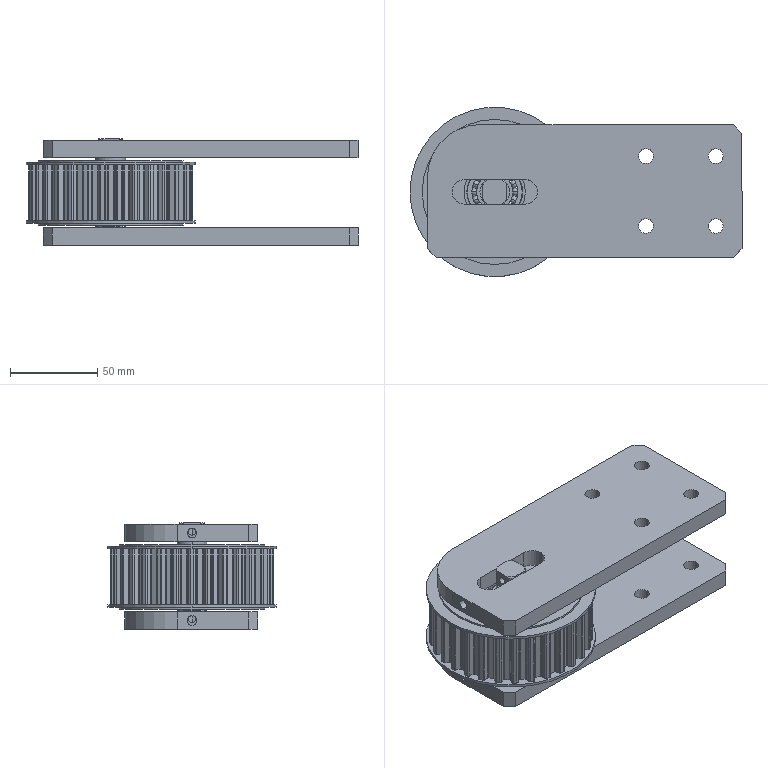Part | SolidWorks | features CompositeCurve 1 | 6 solids | 585 faces | box 190 x 97 x 61 mm | volume 476303 mm3 | cylinder 251 | plane 150 | torus 112 | sphere 64 | cone 8 | commonest cylinder face diameters 1.2 x70 1.6 x70 93.64 x31 8.5 x16 20.667 x8 26.333 x8